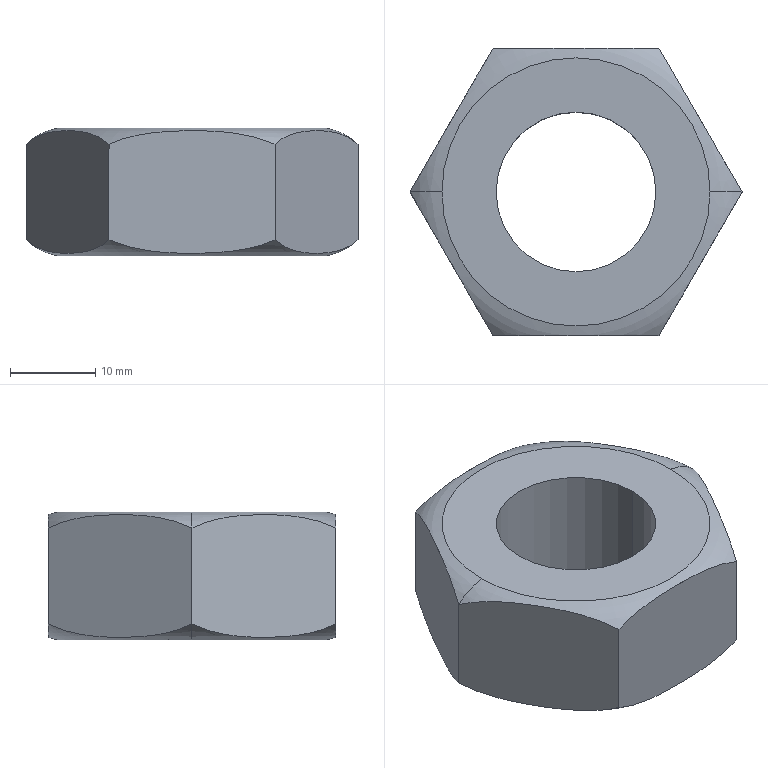Part | SolidWorks | features Extrusion 1, RevCut 1, Scale 1 | 1 solid | 14 faces | box 38.971 x 33.75 x 15 mm | volume 10501 mm3 | plane 8 | torus 4 | cylinder 2 | commonest cylinder face diameters 18.75 x2
STEP:
#1=CARTESIAN_POINT('',(-15.736,-0.00008146,11.5));
#2=VERTEX_POINT('',#1);
#3=CARTESIAN_POINT('',(15.736,-0.00008146,11.5));
#4=VERTEX_POINT('',#3);
#5=CARTESIAN_POINT('',(0.00005689,-0.00008146,11.5));
#6=DIRECTION('',(0.,0.,-1.));
#7=DIRECTION('',(-1.,0.,0.));
#8=AXIS2_PLACEMENT_3D('',#5,#6,#7);
#9=CIRCLE('',#8,15.736);
#10=EDGE_CURVE('',#2,#4,#9,.T.);
#11=ORIENTED_EDGE('',*,*,#10,.T.);
#12=CARTESIAN_POINT('',(19.486,-0.00008146,9.625));
#13=VERTEX_POINT('',#12);
#14=CARTESIAN_POINT('',(14.39,-0.00008146,4.122));
#15=DIRECTION('',(0.,1.,0.));
#16=DIRECTION('',(-1.,0.,0.));
#17=AXIS2_PLACEMENT_3D('',#14,#15,#16);
#18=CIRCLE('',#17,7.5);
#19=EDGE_CURVE('',#4,#13,#18,.T.);
#20=ORIENTED_EDGE('',*,*,#19,.T.);
#21=CARTESIAN_POINT('',(9.743,16.875,9.625));
#22=VERTEX_POINT('',#21);
#23=CARTESIAN_POINT('',(9.743,16.875,9.625));
#24=CARTESIAN_POINT('',(10.123,16.216,9.977));
#25=CARTESIAN_POINT('',(10.516,15.536,10.239));
#26=CARTESIAN_POINT('',(11.316,14.15,10.649));
#27=CARTESIAN_POINT('',(11.724,13.444,10.796));
#28=CARTESIAN_POINT('',(12.549,12.014,11.016));
#29=CARTESIAN_POINT('',(12.962,11.298,11.086));
#30=CARTESIAN_POINT('',(13.788,9.869,11.177));
#31=CARTESIAN_POINT('',(14.2,9.155,11.198));
#32=CARTESIAN_POINT('',(15.024,7.728,11.198));
#33=CARTESIAN_POINT('',(15.436,7.014,11.178));
#34=CARTESIAN_POINT('',(16.259,5.588,11.087));
#35=CARTESIAN_POINT('',(16.671,4.876,11.017));
#36=CARTESIAN_POINT('',(17.493,3.452,10.8));
#37=CARTESIAN_POINT('',(17.905,2.737,10.652));
#38=CARTESIAN_POINT('',(18.711,1.341,10.24));
#39=CARTESIAN_POINT('',(19.105,0.6588,9.977));
#40=CARTESIAN_POINT('',(19.486,-0.00008146,9.625));
#41=B_SPLINE_CURVE_WITH_KNOTS('',3,(#23,#24,#25,#26,#27,#28,#29,#30,#31,#32,#33,#34,#35,#36,#37,#38,#39,#40),.UNSPECIFIED.,.F.,.F.,(4,2,2,2,2,2,2,2,4),(0.00000047,0.002478,0.004956,0.007434,0.009912,0.01239,0.01487,0.01735,0.01982),.UNSPECIFIED.);
#42=EDGE_CURVE('',#22,#13,#41,.T.);
#43=ORIENTED_EDGE('',*,*,#42,.F.);
#44=CARTESIAN_POINT('',(-9.743,16.875,9.625));
#45=VERTEX_POINT('',#44);
#46=CARTESIAN_POINT('',(-9.743,16.875,9.625));
#47=CARTESIAN_POINT('',(-8.991,16.875,9.973));
#48=CARTESIAN_POINT('',(-8.209,16.875,10.235));
#49=CARTESIAN_POINT('',(-7.003,16.875,10.545));
#50=CARTESIAN_POINT('',(-6.595,16.875,10.634));
#51=CARTESIAN_POINT('',(-5.78,16.875,10.787));
#52=CARTESIAN_POINT('',(-5.371,16.875,10.851));
#53=CARTESIAN_POINT('',(-4.142,16.875,11.014));
#54=CARTESIAN_POINT('',(-3.319,16.875,11.085));
#55=CARTESIAN_POINT('',(-1.669,16.875,11.177));
#56=CARTESIAN_POINT('',(-0.841,16.875,11.198));
#57=CARTESIAN_POINT('',(0.8178,16.875,11.198));
#58=CARTESIAN_POINT('',(1.647,16.875,11.178));
#59=CARTESIAN_POINT('',(3.299,16.875,11.087));
#60=CARTESIAN_POINT('',(4.122,16.875,11.016));
#61=CARTESIAN_POINT('',(5.76,16.875,10.8));
#62=CARTESIAN_POINT('',(6.575,16.875,10.654));
#63=CARTESIAN_POINT('',(7.788,16.875,10.344));
#64=CARTESIAN_POINT('',(8.19,16.875,10.226));
#65=CARTESIAN_POINT('',(8.977,16.875,9.954));
#66=CARTESIAN_POINT('',(9.364,16.875,9.8));
#67=CARTESIAN_POINT('',(9.743,16.875,9.625));
#68=B_SPLINE_CURVE_WITH_KNOTS('',3,(#46,#47,#48,#49,#50,#51,#52,#53,#54,#55,#56,#57,#58,#59,#60,#61,#62,#63,#64,#65,#66,#67),.UNSPECIFIED.,.F.,.F.,(4,2,2,2,2,2,2,2,2,2,4),(0.05874,0.06121,0.06245,0.06369,0.06617,0.06865,0.07112,0.0736,0.07608,0.07732,0.07856),.UNSPECIFIED.);
#69=EDGE_CURVE('',#45,#22,#68,.T.);
#70=ORIENTED_EDGE('',*,*,#69,.F.);
#71=CARTESIAN_POINT('',(-19.486,-0.00008146,9.625));
#72=VERTEX_POINT('',#71);
#73=CARTESIAN_POINT('',(-19.486,-0.00008146,9.625));
#74=CARTESIAN_POINT('',(-19.105,0.6591,9.977));
#75=CARTESIAN_POINT('',(-18.712,1.339,10.239));
#76=CARTESIAN_POINT('',(-17.912,2.725,10.649));
#77=CARTESIAN_POINT('',(-17.504,3.431,10.796));
#78=CARTESIAN_POINT('',(-16.679,4.861,11.016));
#79=CARTESIAN_POINT('',(-16.266,5.577,11.086));
#80=CARTESIAN_POINT('',(-15.441,7.006,11.177));
#81=CARTESIAN_POINT('',(-15.029,7.72,11.198));
#82=CARTESIAN_POINT('',(-14.204,9.147,11.198));
#83=CARTESIAN_POINT('',(-13.792,9.861,11.178));
#84=CARTESIAN_POINT('',(-12.969,11.287,11.087));
#85=CARTESIAN_POINT('',(-12.558,11.999,11.017));
#86=CARTESIAN_POINT('',(-11.736,13.423,10.8));
#87=CARTESIAN_POINT('',(-11.323,14.138,10.652));
#88=CARTESIAN_POINT('',(-10.517,15.533,10.24));
#89=CARTESIAN_POINT('',(-10.123,16.216,9.977));
#90=CARTESIAN_POINT('',(-9.743,16.875,9.625));
#91=B_SPLINE_CURVE_WITH_KNOTS('',3,(#73,#74,#75,#76,#77,#78,#79,#80,#81,#82,#83,#84,#85,#86,#87,#88,#89,#90),.UNSPECIFIED.,.F.,.F.,(4,2,2,2,2,2,2,2,4),(0.00000047,0.002478,0.004956,0.007434,0.009912,0.01239,0.01487,0.01735,0.01982),.UNSPECIFIED.);
#92=EDGE_CURVE('',#72,#45,#91,.T.);
#93=ORIENTED_EDGE('',*,*,#92,.F.);
#94=CARTESIAN_POINT('',(-14.39,-0.00008146,4.122));
#95=DIRECTION('',(0.,-1.,0.));
#96=DIRECTION('',(0.,0.,-1.));
#97=AXIS2_PLACEMENT_3D('',#94,#95,#96);
#98=CIRCLE('',#97,7.5);
#99=EDGE_CURVE('',#2,#72,#98,.T.);
#100=ORIENTED_EDGE('',*,*,#99,.F.);
#101=EDGE_LOOP('',(#11,#20,#43,#70,#93,#100));
#102=FACE_OUTER_BOUND('',#101,.T.);
#103=CARTESIAN_POINT('',(0.00005689,-0.00008146,4.122));
#104=DIRECTION('',(0.,0.,-1.));
#105=DIRECTION('',(-1.,0.,0.));
#106=AXIS2_PLACEMENT_3D('',#103,#104,#105);
#107=TOROIDAL_SURFACE('',#106,14.39,7.5);
#108=ADVANCED_FACE('',(#102),#107,.T.);
#109=CARTESIAN_POINT('',(19.486,-0.00008146,-1.625));
#110=VERTEX_POINT('',#109);
#111=CARTESIAN_POINT('',(9.743,16.875,-1.625));
#112=VERTEX_POINT('',#111);
#113=CARTESIAN_POINT('',(19.486,-0.00008146,-1.625));
#114=CARTESIAN_POINT('',(19.105,0.6591,-1.977));
#115=CARTESIAN_POINT('',(18.712,1.339,-2.239));
#116=CARTESIAN_POINT('',(17.912,2.725,-2.649));
#117=CARTESIAN_POINT('',(17.505,3.431,-2.796));
#118=CARTESIAN_POINT('',(16.679,4.861,-3.016));
#119=CARTESIAN_POINT('',(16.266,5.577,-3.086));
#120=CARTESIAN_POINT('',(15.441,7.006,-3.177));
#121=CARTESIAN_POINT('',(15.029,7.72,-3.198));
#122=CARTESIAN_POINT('',(14.204,9.147,-3.198));
#123=CARTESIAN_POINT('',(13.793,9.861,-3.178));
#124=CARTESIAN_POINT('',(12.969,11.287,-3.087));
#125=CARTESIAN_POINT('',(12.558,11.999,-3.017));
#126=CARTESIAN_POINT('',(11.736,13.423,-2.8));
#127=CARTESIAN_POINT('',(11.323,14.138,-2.652));
#128=CARTESIAN_POINT('',(10.517,15.533,-2.24));
#129=CARTESIAN_POINT('',(10.123,16.216,-1.977));
#130=CARTESIAN_POINT('',(9.743,16.875,-1.625));
#131=B_SPLINE_CURVE_WITH_KNOTS('',3,(#113,#114,#115,#116,#117,#118,#119,#120,#121,#122,#123,#124,#125,#126,#127,#128,#129,#130),.UNSPECIFIED.,.F.,.F.,(4,2,2,2,2,2,2,2,4),(0.00000047,0.002478,0.004956,0.007434,0.009912,0.01239,0.01487,0.01735,0.01982),.UNSPECIFIED.);
#132=EDGE_CURVE('',#110,#112,#131,.T.);
#133=ORIENTED_EDGE('',*,*,#132,.F.);
#134=CARTESIAN_POINT('',(15.736,-0.00008146,-3.5));
#135=VERTEX_POINT('',#134);
#136=CARTESIAN_POINT('',(14.39,-0.00008146,3.878));
#137=DIRECTION('',(0.,1.,0.));
#138=DIRECTION('',(-1.,0.,0.));
#139=AXIS2_PLACEMENT_3D('',#136,#137,#138);
#140=CIRCLE('',#139,7.5);
#141=EDGE_CURVE('',#110,#135,#140,.T.);
#142=ORIENTED_EDGE('',*,*,#141,.T.);
#143=CARTESIAN_POINT('',(-15.736,-0.00008146,-3.5));
#144=VERTEX_POINT('',#143);
#145=CARTESIAN_POINT('',(0.00005689,-0.00008146,-3.5));
#146=DIRECTION('',(0.,0.,-1.));
#147=DIRECTION('',(-1.,0.,0.));
#148=AXIS2_PLACEMENT_3D('',#145,#146,#147);
#149=CIRCLE('',#148,15.736);
#150=EDGE_CURVE('',#144,#135,#149,.T.);
#151=ORIENTED_EDGE('',*,*,#150,.F.);
#152=CARTESIAN_POINT('',(-19.486,-0.00008146,-1.625));
#153=VERTEX_POINT('',#152);
#154=CARTESIAN_POINT('',(-14.39,-0.00008146,3.878));
#155=DIRECTION('',(0.,-1.,0.));
#156=DIRECTION('',(0.,0.,-1.));
#157=AXIS2_PLACEMENT_3D('',#154,#155,#156);
#158=CIRCLE('',#157,7.5);
#159=EDGE_CURVE('',#153,#144,#158,.T.);
#160=ORIENTED_EDGE('',*,*,#159,.F.);
#161=CARTESIAN_POINT('',(-9.743,16.875,-1.625));
#162=VERTEX_POINT('',#161);
#163=CARTESIAN_POINT('',(-9.743,16.875,-1.625));
#164=CARTESIAN_POINT('',(-10.123,16.216,-1.977));
#165=CARTESIAN_POINT('',(-10.516,15.536,-2.239));
#166=CARTESIAN_POINT('',(-11.316,14.15,-2.649));
#167=CARTESIAN_POINT('',(-11.724,13.444,-2.796));
#168=CARTESIAN_POINT('',(-12.549,12.014,-3.016));
#169=CARTESIAN_POINT('',(-12.962,11.298,-3.086));
#170=CARTESIAN_POINT('',(-13.787,9.869,-3.177));
#171=CARTESIAN_POINT('',(-14.2,9.155,-3.198));
#172=CARTESIAN_POINT('',(-15.024,7.728,-3.198));
#173=CARTESIAN_POINT('',(-15.436,7.014,-3.178));
#174=CARTESIAN_POINT('',(-16.259,5.588,-3.087));
#175=CARTESIAN_POINT('',(-16.67,4.876,-3.017));
#176=CARTESIAN_POINT('',(-17.492,3.452,-2.8));
#177=CARTESIAN_POINT('',(-17.905,2.737,-2.652));
#178=CARTESIAN_POINT('',(-18.711,1.341,-2.24));
#179=CARTESIAN_POINT('',(-19.105,0.6588,-1.977));
#180=CARTESIAN_POINT('',(-19.486,-0.00008146,-1.625));
#181=B_SPLINE_CURVE_WITH_KNOTS('',3,(#163,#164,#165,#166,#167,#168,#169,#170,#171,#172,#173,#174,#175,#176,#177,#178,#179,#180),.UNSPECIFIED.,.F.,.F.,(4,2,2,2,2,2,2,2,4),(0.00000047,0.002478,0.004956,0.007434,0.009912,0.01239,0.01487,0.01735,0.01982),.UNSPECIFIED.);
#182=EDGE_CURVE('',#162,#153,#181,.T.);
#183=ORIENTED_EDGE('',*,*,#182,.F.);
#184=CARTESIAN_POINT('',(9.743,16.875,-1.625));
#185=CARTESIAN_POINT('',(8.992,16.875,-1.973));
#186=CARTESIAN_POINT('',(8.209,16.875,-2.235));
#187=CARTESIAN_POINT('',(7.003,16.875,-2.545));
#188=CARTESIAN_POINT('',(6.596,16.875,-2.634));
#189=CARTESIAN_POINT('',(5.78,16.875,-2.786));
#190=CARTESIAN_POINT('',(5.371,16.875,-2.851));
#191=CARTESIAN_POINT('',(4.142,16.875,-3.014));
#192=CARTESIAN_POINT('',(3.319,16.875,-3.085));
#193=CARTESIAN_POINT('',(1.669,16.875,-3.177));
#194=CARTESIAN_POINT('',(0.8411,16.875,-3.198));
#195=CARTESIAN_POINT('',(-0.8176,16.875,-3.198));
#196=CARTESIAN_POINT('',(-1.647,16.875,-3.178));
#197=CARTESIAN_POINT('',(-3.299,16.875,-3.087));
#198=CARTESIAN_POINT('',(-4.122,16.875,-3.016));
#199=CARTESIAN_POINT('',(-5.76,16.875,-2.8));
#200=CARTESIAN_POINT('',(-6.575,16.875,-2.654));
#201=CARTESIAN_POINT('',(-7.788,16.875,-2.344));
#202=CARTESIAN_POINT('',(-8.189,16.875,-2.226));
#203=CARTESIAN_POINT('',(-8.977,16.875,-1.954));
#204=CARTESIAN_POINT('',(-9.364,16.875,-1.8));
#205=CARTESIAN_POINT('',(-9.743,16.875,-1.625));
#206=B_SPLINE_CURVE_WITH_KNOTS('',3,(#184,#185,#186,#187,#188,#189,#190,#191,#192,#193,#194,#195,#196,#197,#198,#199,#200,#201,#202,#203,#204,#205),.UNSPECIFIED.,.F.,.F.,(4,2,2,2,2,2,2,2,2,2,4),(0.05874,0.06121,0.06245,0.06369,0.06617,0.06865,0.07112,0.0736,0.07608,0.07732,0.07856),.UNSPECIFIED.);
#207=EDGE_CURVE('',#112,#162,#206,.T.);
#208=ORIENTED_EDGE('',*,*,#207,.F.);
#209=EDGE_LOOP('',(#133,#142,#151,#160,#183,#208));
#210=FACE_OUTER_BOUND('',#209,.T.);
#211=CARTESIAN_POINT('',(0.00005689,-0.00008146,3.878));
#212=DIRECTION('',(0.,0.,-1.));
#213=DIRECTION('',(-1.,0.,0.));
#214=AXIS2_PLACEMENT_3D('',#211,#212,#213);
#215=TOROIDAL_SURFACE('',#214,14.39,7.5);
#216=ADVANCED_FACE('',(#210),#215,.T.);
#217=CARTESIAN_POINT('',(-9.375,-0.00008146,11.5));
#218=VERTEX_POINT('',#217);
#219=CARTESIAN_POINT('',(9.375,-0.00008146,11.5));
#220=VERTEX_POINT('',#219);
#221=CARTESIAN_POINT('',(0.00005689,-0.00008146,11.5));
#222=DIRECTION('',(0.,0.,1.));
#223=DIRECTION('',(1.,0.,0.));
#224=AXIS2_PLACEMENT_3D('',#221,#222,#223);
#225=CIRCLE('',#224,9.375);
#226=EDGE_CURVE('',#218,#220,#225,.T.);
#227=ORIENTED_EDGE('',*,*,#226,.T.);
#228=CARTESIAN_POINT('',(9.375,-0.00008146,-3.5));
#229=VERTEX_POINT('',#228);
#230=CARTESIAN_POINT('',(9.375,-0.00008146,11.5));
#231=DIRECTION('',(0.,0.,-1.));
#232=VECTOR('',#231,1000.);
#233=LINE('',#230,#232);
#234=EDGE_CURVE('',#220,#229,#233,.T.);
#235=ORIENTED_EDGE('',*,*,#234,.T.);
#236=CARTESIAN_POINT('',(-9.375,-0.00008146,-3.5));
#237=VERTEX_POINT('',#236);
#238=CARTESIAN_POINT('',(0.00005689,-0.00008146,-3.5));
#239=DIRECTION('',(0.,0.,1.));
#240=DIRECTION('',(1.,0.,0.));
#241=AXIS2_PLACEMENT_3D('',#238,#239,#240);
#242=CIRCLE('',#241,9.375);
#243=EDGE_CURVE('',#237,#229,#242,.T.);
#244=ORIENTED_EDGE('',*,*,#243,.F.);
#245=CARTESIAN_POINT('',(-9.375,-0.00008146,11.5));
#246=DIRECTION('',(0.,0.,-1.));
#247=VECTOR('',#246,1000.);
#248=LINE('',#245,#247);
#249=EDGE_CURVE('',#218,#237,#248,.T.);
#250=ORIENTED_EDGE('',*,*,#249,.F.);
#251=EDGE_LOOP('',(#227,#235,#244,#250));
#252=FACE_OUTER_BOUND('',#251,.T.);
#253=CARTESIAN_POINT('',(0.00005689,-0.00008146,11.5));
#254=DIRECTION('',(0.,0.,-1.));
#255=DIRECTION('',(-1.,0.,0.));
#256=AXIS2_PLACEMENT_3D('',#253,#254,#255);
#257=CYLINDRICAL_SURFACE('',#256,9.375);
#258=ADVANCED_FACE('',(#252),#257,.F.);
#259=ORIENTED_EDGE('',*,*,#10,.F.);
#260=CARTESIAN_POINT('',(0.00005689,-0.00008146,11.5));
#261=DIRECTION('',(0.,0.,-1.));
#262=DIRECTION('',(-1.,0.,0.));
#263=AXIS2_PLACEMENT_3D('',#260,#261,#262);
#264=CIRCLE('',#263,15.736);
#265=EDGE_CURVE('',#4,#2,#264,.T.);
#266=ORIENTED_EDGE('',*,*,#265,.F.);
#267=EDGE_LOOP('',(#259,#266));
#268=FACE_OUTER_BOUND('',#267,.T.);
#269=ORIENTED_EDGE('',*,*,#226,.F.);
#270=CARTESIAN_POINT('',(0.00005689,-0.00008146,11.5));
#271=DIRECTION('',(0.,0.,1.));
#272=DIRECTION('',(1.,0.,0.));
#273=AXIS2_PLACEMENT_3D('',#270,#271,#272);
#274=CIRCLE('',#273,9.375);
#275=EDGE_CURVE('',#220,#218,#274,.T.);
#276=ORIENTED_EDGE('',*,*,#275,.F.);
#277=EDGE_LOOP('',(#269,#276));
#278=FACE_BOUND('',#277,.T.);
#279=CARTESIAN_POINT('',(0.00005689,-0.00008146,11.5));
#280=DIRECTION('',(0.,0.,1.));
#281=DIRECTION('',(1.,0.,0.));
#282=AXIS2_PLACEMENT_3D('',#279,#280,#281);
#283=PLANE('',#282);
#284=ADVANCED_FACE('',(#268,#278),#283,.T.);
#285=ORIENTED_EDGE('',*,*,#150,.T.);
#286=CARTESIAN_POINT('',(0.00005689,-0.00008146,-3.5));
#287=DIRECTION('',(0.,0.,-1.));
#288=DIRECTION('',(-1.,0.,0.));
#289=AXIS2_PLACEMENT_3D('',#286,#287,#288);
#290=CIRCLE('',#289,15.736);
#291=EDGE_CURVE('',#135,#144,#290,.T.);
#292=ORIENTED_EDGE('',*,*,#291,.T.);
#293=EDGE_LOOP('',(#285,#292));
#294=FACE_OUTER_BOUND('',#293,.T.);
#295=ORIENTED_EDGE('',*,*,#243,.T.);
#296=CARTESIAN_POINT('',(0.00005689,-0.00008146,-3.5));
#297=DIRECTION('',(0.,0.,1.));
#298=DIRECTION('',(1.,0.,0.));
#299=AXIS2_PLACEMENT_3D('',#296,#297,#298);
#300=CIRCLE('',#299,9.375);
#301=EDGE_CURVE('',#229,#237,#300,.T.);
#302=ORIENTED_EDGE('',*,*,#301,.T.);
#303=EDGE_LOOP('',(#295,#302));
#304=FACE_BOUND('',#303,.T.);
#305=CARTESIAN_POINT('',(0.00005689,-0.00008146,-3.5));
#306=DIRECTION('',(0.,0.,1.));
#307=DIRECTION('',(1.,0.,0.));
#308=AXIS2_PLACEMENT_3D('',#305,#306,#307);
#309=PLANE('',#308);
#310=ADVANCED_FACE('',(#294,#304),#309,.F.);
#311=CARTESIAN_POINT('',(19.486,-0.00008146,11.5));
#312=DIRECTION('',(0.,0.,-1.));
#313=VECTOR('',#312,1000.);
#314=LINE('',#311,#313);
#315=EDGE_CURVE('',#13,#110,#314,.T.);
#316=ORIENTED_EDGE('',*,*,#315,.F.);
#317=CARTESIAN_POINT('',(9.743,-16.875,9.625));
#318=VERTEX_POINT('',#317);
#319=CARTESIAN_POINT('',(19.486,-0.00008146,9.625));
#320=CARTESIAN_POINT('',(19.105,-0.6593,9.977));
#321=CARTESIAN_POINT('',(18.712,-1.339,10.239));
#322=CARTESIAN_POINT('',(17.912,-2.725,10.649));
#323=CARTESIAN_POINT('',(17.505,-3.431,10.796));
#324=CARTESIAN_POINT('',(16.679,-4.861,11.016));
#325=CARTESIAN_POINT('',(16.266,-5.577,11.086));
#326=CARTESIAN_POINT('',(15.441,-7.006,11.177));
#327=CARTESIAN_POINT('',(15.029,-7.72,11.198));
#328=CARTESIAN_POINT('',(14.204,-9.147,11.198));
#329=CARTESIAN_POINT('',(13.793,-9.861,11.178));
#330=CARTESIAN_POINT('',(12.969,-11.287,11.087));
#331=CARTESIAN_POINT('',(12.558,-11.999,11.017));
#332=CARTESIAN_POINT('',(11.736,-13.423,10.8));
#333=CARTESIAN_POINT('',(11.323,-14.138,10.652));
#334=CARTESIAN_POINT('',(10.517,-15.534,10.24));
#335=CARTESIAN_POINT('',(10.123,-16.216,9.977));
#336=CARTESIAN_POINT('',(9.743,-16.875,9.625));
#337=B_SPLINE_CURVE_WITH_KNOTS('',3,(#319,#320,#321,#322,#323,#324,#325,#326,#327,#328,#329,#330,#331,#332,#333,#334,#335,#336),.UNSPECIFIED.,.F.,.F.,(4,2,2,2,2,2,2,2,4),(0.00000047,0.002478,0.004956,0.007434,0.009912,0.01239,0.01487,0.01735,0.01982),.UNSPECIFIED.);
#338=EDGE_CURVE('',#13,#318,#337,.T.);
#339=ORIENTED_EDGE('',*,*,#338,.T.);
#340=CARTESIAN_POINT('',(9.743,-16.875,-1.625));
#341=VERTEX_POINT('',#340);
#342=CARTESIAN_POINT('',(9.743,-16.875,11.5));
#343=DIRECTION('',(0.,0.,-1.));
#344=VECTOR('',#343,1000.);
#345=LINE('',#342,#344);
#346=EDGE_CURVE('',#318,#341,#345,.T.);
#347=ORIENTED_EDGE('',*,*,#346,.T.);
#348=CARTESIAN_POINT('',(9.743,-16.875,-1.625));
#349=CARTESIAN_POINT('',(10.123,-16.216,-1.977));
#350=CARTESIAN_POINT('',(10.516,-15.536,-2.239));
#351=CARTESIAN_POINT('',(11.316,-14.15,-2.649));
#352=CARTESIAN_POINT('',(11.724,-13.444,-2.796));
#353=CARTESIAN_POINT('',(12.549,-12.014,-3.016));
#354=CARTESIAN_POINT('',(12.962,-11.298,-3.086));
#355=CARTESIAN_POINT('',(13.788,-9.869,-3.177));
#356=CARTESIAN_POINT('',(14.2,-9.155,-3.198));
#357=CARTESIAN_POINT('',(15.024,-7.728,-3.198));
#358=CARTESIAN_POINT('',(15.436,-7.014,-3.178));
#359=CARTESIAN_POINT('',(16.259,-5.588,-3.087));
#360=CARTESIAN_POINT('',(16.671,-4.876,-3.017));
#361=CARTESIAN_POINT('',(17.493,-3.452,-2.8));
#362=CARTESIAN_POINT('',(17.905,-2.737,-2.652));
#363=CARTESIAN_POINT('',(18.711,-1.342,-2.24));
#364=CARTESIAN_POINT('',(19.105,-0.659,-1.977));
#365=CARTESIAN_POINT('',(19.486,-0.00008146,-1.625));
#366=B_SPLINE_CURVE_WITH_KNOTS('',3,(#348,#349,#350,#351,#352,#353,#354,#355,#356,#357,#358,#359,#360,#361,#362,#363,#364,#365),.UNSPECIFIED.,.F.,.F.,(4,2,2,2,2,2,2,2,4),(0.00000047,0.002478,0.004956,0.007434,0.009912,0.01239,0.01487,0.01735,0.01982),.UNSPECIFIED.);
#367=EDGE_CURVE('',#341,#110,#366,.T.);
#368=ORIENTED_EDGE('',*,*,#367,.T.);
#369=EDGE_LOOP('',(#316,#339,#347,#368));
#370=FACE_OUTER_BOUND('',#369,.T.);
#371=CARTESIAN_POINT('',(9.743,-16.875,11.5));
#372=DIRECTION('',(-0.866,0.5,0.));
#373=DIRECTION('',(-0.5,-0.866,0.));
#374=AXIS2_PLACEMENT_3D('',#371,#372,#373);
#375=PLANE('',#374);
#376=ADVANCED_FACE('',(#370),#375,.F.);
#377=CARTESIAN_POINT('',(9.743,16.875,11.5));
#378=DIRECTION('',(0.,0.,-1.));
#379=VECTOR('',#378,1000.);
#380=LINE('',#377,#379);
#381=EDGE_CURVE('',#22,#112,#380,.T.);
#382=ORIENTED_EDGE('',*,*,#381,.F.);
#383=ORIENTED_EDGE('',*,*,#42,.T.);
#384=ORIENTED_EDGE('',*,*,#315,.T.);
#385=ORIENTED_EDGE('',*,*,#132,.T.);
#386=EDGE_LOOP('',(#382,#383,#384,#385));
#387=FACE_OUTER_BOUND('',#386,.T.);
#388=CARTESIAN_POINT('',(19.486,-0.00008146,11.5));
#389=DIRECTION('',(-0.866,-0.5,0.));
#390=DIRECTION('',(0.5,-0.866,0.));
#391=AXIS2_PLACEMENT_3D('',#388,#389,#390);
#392=PLANE('',#391);
#393=ADVANCED_FACE('',(#387),#392,.F.);
#394=CARTESIAN_POINT('',(-9.743,16.875,11.5));
#395=DIRECTION('',(0.,0.,-1.));
#396=VECTOR('',#395,1000.);
#397=LINE('',#394,#396);
#398=EDGE_CURVE('',#45,#162,#397,.T.);
#399=ORIENTED_EDGE('',*,*,#398,.F.);
#400=ORIENTED_EDGE('',*,*,#69,.T.);
#401=ORIENTED_EDGE('',*,*,#381,.T.);
#402=ORIENTED_EDGE('',*,*,#207,.T.);
#403=EDGE_LOOP('',(#399,#400,#401,#402));
#404=FACE_OUTER_BOUND('',#403,.T.);
#405=CARTESIAN_POINT('',(9.743,16.875,11.5));
#406=DIRECTION('',(0.,-1.,0.));
#407=DIRECTION('',(0.,0.,-1.));
#408=AXIS2_PLACEMENT_3D('',#405,#406,#407);
#409=PLANE('',#408);
#410=ADVANCED_FACE('',(#404),#409,.F.);
#411=CARTESIAN_POINT('',(-19.486,-0.00008146,11.5));
#412=DIRECTION('',(0.,0.,-1.));
#413=VECTOR('',#412,1000.);
#414=LINE('',#411,#413);
#415=EDGE_CURVE('',#72,#153,#414,.T.);
#416=ORIENTED_EDGE('',*,*,#415,.F.);
#417=ORIENTED_EDGE('',*,*,#92,.T.);
#418=ORIENTED_EDGE('',*,*,#398,.T.);
#419=ORIENTED_EDGE('',*,*,#182,.T.);
#420=EDGE_LOOP('',(#416,#417,#418,#419));
#421=FACE_OUTER_BOUND('',#420,.T.);
#422=CARTESIAN_POINT('',(-9.743,16.875,11.5));
#423=DIRECTION('',(0.866,-0.5,0.));
#424=DIRECTION('',(0.5,0.866,0.));
#425=AXIS2_PLACEMENT_3D('',#422,#423,#424);
#426=PLANE('',#425);
#427=ADVANCED_FACE('',(#421),#426,.F.);
#428=CARTESIAN_POINT('',(-9.743,-16.875,9.625));
#429=VERTEX_POINT('',#428);
#430=CARTESIAN_POINT('',(-9.743,-16.875,-1.625));
#431=VERTEX_POINT('',#430);
#432=CARTESIAN_POINT('',(-9.743,-16.875,11.5));
#433=DIRECTION('',(0.,0.,-1.));
#434=VECTOR('',#433,1000.);
#435=LINE('',#432,#434);
#436=EDGE_CURVE('',#429,#431,#435,.T.);
#437=ORIENTED_EDGE('',*,*,#436,.F.);
#438=CARTESIAN_POINT('',(-9.743,-16.875,9.625));
#439=CARTESIAN_POINT('',(-10.123,-16.216,9.977));
#440=CARTESIAN_POINT('',(-10.516,-15.536,10.239));
#441=CARTESIAN_POINT('',(-11.316,-14.15,10.649));
#442=CARTESIAN_POINT('',(-11.724,-13.444,10.796));
#443=CARTESIAN_POINT('',(-12.549,-12.014,11.016));
#444=CARTESIAN_POINT('',(-12.962,-11.298,11.086));
#445=CARTESIAN_POINT('',(-13.787,-9.869,11.177));
#446=CARTESIAN_POINT('',(-14.2,-9.155,11.198));
#447=CARTESIAN_POINT('',(-15.024,-7.728,11.198));
#448=CARTESIAN_POINT('',(-15.436,-7.014,11.178));
#449=CARTESIAN_POINT('',(-16.259,-5.588,11.087));
#450=CARTESIAN_POINT('',(-16.67,-4.876,11.017));
#451=CARTESIAN_POINT('',(-17.492,-3.452,10.8));
#452=CARTESIAN_POINT('',(-17.905,-2.737,10.652));
#453=CARTESIAN_POINT('',(-18.711,-1.342,10.24));
#454=CARTESIAN_POINT('',(-19.105,-0.659,9.977));
#455=CARTESIAN_POINT('',(-19.486,-0.00008146,9.625));
#456=B_SPLINE_CURVE_WITH_KNOTS('',3,(#438,#439,#440,#441,#442,#443,#444,#445,#446,#447,#448,#449,#450,#451,#452,#453,#454,#455),.UNSPECIFIED.,.F.,.F.,(4,2,2,2,2,2,2,2,4),(0.00000047,0.002478,0.004956,0.007434,0.009912,0.01239,0.01487,0.01735,0.01982),.UNSPECIFIED.);
#457=EDGE_CURVE('',#429,#72,#456,.T.);
#458=ORIENTED_EDGE('',*,*,#457,.T.);
#459=ORIENTED_EDGE('',*,*,#415,.T.);
#460=CARTESIAN_POINT('',(-19.486,-0.00008146,-1.625));
#461=CARTESIAN_POINT('',(-19.105,-0.6593,-1.977));
#462=CARTESIAN_POINT('',(-18.712,-1.339,-2.239));
#463=CARTESIAN_POINT('',(-17.912,-2.725,-2.649));
#464=CARTESIAN_POINT('',(-17.504,-3.431,-2.796));
#465=CARTESIAN_POINT('',(-16.679,-4.861,-3.016));
#466=CARTESIAN_POINT('',(-16.266,-5.577,-3.086));
#467=CARTESIAN_POINT('',(-15.441,-7.006,-3.177));
#468=CARTESIAN_POINT('',(-15.029,-7.72,-3.198));
#469=CARTESIAN_POINT('',(-14.204,-9.147,-3.198));
#470=CARTESIAN_POINT('',(-13.792,-9.861,-3.178));
#471=CARTESIAN_POINT('',(-12.969,-11.287,-3.087));
#472=CARTESIAN_POINT('',(-12.558,-11.999,-3.017));
#473=CARTESIAN_POINT('',(-11.736,-13.423,-2.8));
#474=CARTESIAN_POINT('',(-11.323,-14.138,-2.652));
#475=CARTESIAN_POINT('',(-10.517,-15.534,-2.24));
#476=CARTESIAN_POINT('',(-10.123,-16.216,-1.977));
#477=CARTESIAN_POINT('',(-9.743,-16.875,-1.625));
#478=B_SPLINE_CURVE_WITH_KNOTS('',3,(#460,#461,#462,#463,#464,#465,#466,#467,#468,#469,#470,#471,#472,#473,#474,#475,#476,#477),.UNSPECIFIED.,.F.,.F.,(4,2,2,2,2,2,2,2,4),(0.00000047,0.002478,0.004956,0.007434,0.009912,0.01239,0.01487,0.01735,0.01982),.UNSPECIFIED.);
#479=EDGE_CURVE('',#153,#431,#478,.T.);
#480=ORIENTED_EDGE('',*,*,#479,.T.);
#481=EDGE_LOOP('',(#437,#458,#459,#480));
#482=FACE_OUTER_BOUND('',#481,.T.);
#483=CARTESIAN_POINT('',(-19.486,-0.00008146,11.5));
#484=DIRECTION('',(0.866,0.5,0.));
#485=DIRECTION('',(-0.5,0.866,0.));
#486=AXIS2_PLACEMENT_3D('',#483,#484,#485);
#487=PLANE('',#486);
#488=ADVANCED_FACE('',(#482),#487,.F.);
#489=ORIENTED_EDGE('',*,*,#346,.F.);
#490=CARTESIAN_POINT('',(9.743,-16.875,9.625));
#491=CARTESIAN_POINT('',(8.992,-16.875,9.973));
#492=CARTESIAN_POINT('',(8.209,-16.875,10.235));
#493=CARTESIAN_POINT('',(7.003,-16.875,10.545));
#494=CARTESIAN_POINT('',(6.596,-16.875,10.634));
#495=CARTESIAN_POINT('',(5.78,-16.875,10.787));
#496=CARTESIAN_POINT('',(5.371,-16.875,10.851));
#497=CARTESIAN_POINT('',(4.142,-16.875,11.014));
#498=CARTESIAN_POINT('',(3.319,-16.875,11.085));
#499=CARTESIAN_POINT('',(1.669,-16.875,11.177));
#500=CARTESIAN_POINT('',(0.8411,-16.875,11.198));
#501=CARTESIAN_POINT('',(-0.8176,-16.875,11.198));
#502=CARTESIAN_POINT('',(-1.647,-16.875,11.178));
#503=CARTESIAN_POINT('',(-3.299,-16.875,11.087));
#504=CARTESIAN_POINT('',(-4.122,-16.875,11.016));
#505=CARTESIAN_POINT('',(-5.76,-16.875,10.8));
#506=CARTESIAN_POINT('',(-6.575,-16.875,10.654));
#507=CARTESIAN_POINT('',(-7.788,-16.875,10.344));
#508=CARTESIAN_POINT('',(-8.189,-16.875,10.226));
#509=CARTESIAN_POINT('',(-8.977,-16.875,9.954));
#510=CARTESIAN_POINT('',(-9.364,-16.875,9.8));
#511=CARTESIAN_POINT('',(-9.743,-16.875,9.625));
#512=B_SPLINE_CURVE_WITH_KNOTS('',3,(#490,#491,#492,#493,#494,#495,#496,#497,#498,#499,#500,#501,#502,#503,#504,#505,#506,#507,#508,#509,#510,#511),.UNSPECIFIED.,.F.,.F.,(4,2,2,2,2,2,2,2,2,2,4),(0.05874,0.06121,0.06245,0.06369,0.06617,0.06865,0.07112,0.0736,0.07608,0.07732,0.07856),.UNSPECIFIED.);
#513=EDGE_CURVE('',#318,#429,#512,.T.);
#514=ORIENTED_EDGE('',*,*,#513,.T.);
#515=ORIENTED_EDGE('',*,*,#436,.T.);
#516=CARTESIAN_POINT('',(-9.743,-16.875,-1.625));
#517=CARTESIAN_POINT('',(-8.991,-16.875,-1.973));
#518=CARTESIAN_POINT('',(-8.209,-16.875,-2.235));
#519=CARTESIAN_POINT('',(-7.003,-16.875,-2.545));
#520=CARTESIAN_POINT('',(-6.595,-16.875,-2.634));
#521=CARTESIAN_POINT('',(-5.78,-16.875,-2.786));
#522=CARTESIAN_POINT('',(-5.371,-16.875,-2.851));
#523=CARTESIAN_POINT('',(-4.142,-16.875,-3.014));
#524=CARTESIAN_POINT('',(-3.319,-16.875,-3.085));
#525=CARTESIAN_POINT('',(-1.669,-16.875,-3.177));
#526=CARTESIAN_POINT('',(-0.841,-16.875,-3.198));
#527=CARTESIAN_POINT('',(0.8178,-16.875,-3.198));
#528=CARTESIAN_POINT('',(1.647,-16.875,-3.178));
#529=CARTESIAN_POINT('',(3.299,-16.875,-3.087));
#530=CARTESIAN_POINT('',(4.122,-16.875,-3.016));
#531=CARTESIAN_POINT('',(5.76,-16.875,-2.8));
#532=CARTESIAN_POINT('',(6.575,-16.875,-2.654));
#533=CARTESIAN_POINT('',(7.788,-16.875,-2.344));
#534=CARTESIAN_POINT('',(8.19,-16.875,-2.226));
#535=CARTESIAN_POINT('',(8.977,-16.875,-1.954));
#536=CARTESIAN_POINT('',(9.364,-16.875,-1.8));
#537=CARTESIAN_POINT('',(9.743,-16.875,-1.625));
#538=B_SPLINE_CURVE_WITH_KNOTS('',3,(#516,#517,#518,#519,#520,#521,#522,#523,#524,#525,#526,#527,#528,#529,#530,#531,#532,#533,#534,#535,#536,#537),.UNSPECIFIED.,.F.,.F.,(4,2,2,2,2,2,2,2,2,2,4),(0.05874,0.06121,0.06245,0.06369,0.06617,0.06865,0.07112,0.0736,0.07608,0.07732,0.07856),.UNSPECIFIED.);
#539=EDGE_CURVE('',#431,#341,#538,.T.);
#540=ORIENTED_EDGE('',*,*,#539,.T.);
#541=EDGE_LOOP('',(#489,#514,#515,#540));
#542=FACE_OUTER_BOUND('',#541,.T.);
#543=CARTESIAN_POINT('',(-9.743,-16.875,11.5));
#544=DIRECTION('',(0.,1.,0.));
#545=DIRECTION('',(-1.,0.,0.));
#546=AXIS2_PLACEMENT_3D('',#543,#544,#545);
#547=PLANE('',#546);
#548=ADVANCED_FACE('',(#542),#547,.F.);
#549=ORIENTED_EDGE('',*,*,#234,.F.);
#550=ORIENTED_EDGE('',*,*,#275,.T.);
#551=ORIENTED_EDGE('',*,*,#249,.T.);
#552=ORIENTED_EDGE('',*,*,#301,.F.);
#553=EDGE_LOOP('',(#549,#550,#551,#552));
#554=FACE_OUTER_BOUND('',#553,.T.);
#555=CARTESIAN_POINT('',(0.00005689,-0.00008146,11.5));
#556=DIRECTION('',(0.,0.,-1.));
#557=DIRECTION('',(-1.,0.,0.));
#558=AXIS2_PLACEMENT_3D('',#555,#556,#557);
#559=CYLINDRICAL_SURFACE('',#558,9.375);
#560=ADVANCED_FACE('',(#554),#559,.F.);
#561=ORIENTED_EDGE('',*,*,#141,.F.);
#562=ORIENTED_EDGE('',*,*,#367,.F.);
#563=ORIENTED_EDGE('',*,*,#539,.F.);
#564=ORIENTED_EDGE('',*,*,#479,.F.);
#565=ORIENTED_EDGE('',*,*,#159,.T.);
#566=ORIENTED_EDGE('',*,*,#291,.F.);
#567=EDGE_LOOP('',(#561,#562,#563,#564,#565,#566));
#568=FACE_OUTER_BOUND('',#567,.T.);
#569=CARTESIAN_POINT('',(0.00005689,-0.00008146,3.878));
#570=DIRECTION('',(0.,0.,-1.));
#571=DIRECTION('',(-1.,0.,0.));
#572=AXIS2_PLACEMENT_3D('',#569,#570,#571);
#573=TOROIDAL_SURFACE('',#572,14.39,7.5);
#574=ADVANCED_FACE('',(#568),#573,.T.);
#575=ORIENTED_EDGE('',*,*,#19,.F.);
#576=ORIENTED_EDGE('',*,*,#265,.T.);
#577=ORIENTED_EDGE('',*,*,#99,.T.);
#578=ORIENTED_EDGE('',*,*,#457,.F.);
#579=ORIENTED_EDGE('',*,*,#513,.F.);
#580=ORIENTED_EDGE('',*,*,#338,.F.);
#581=EDGE_LOOP('',(#575,#576,#577,#578,#579,#580));
#582=FACE_OUTER_BOUND('',#581,.T.);
#583=CARTESIAN_POINT('',(0.00005689,-0.00008146,4.122));
#584=DIRECTION('',(0.,0.,-1.));
#585=DIRECTION('',(-1.,0.,0.));
#586=AXIS2_PLACEMENT_3D('',#583,#584,#585);
#587=TOROIDAL_SURFACE('',#586,14.39,7.5);
#588=ADVANCED_FACE('',(#582),#587,.T.);
#589=CLOSED_SHELL('',(#108,#216,#258,#284,#310,#376,#393,#410,#427,#488,#548,#560,#574,#588));
#590=MANIFOLD_SOLID_BREP('',#589);
#591=CARTESIAN_POINT('',(0.,0.,0.));
#592=DIRECTION('',(0.,0.,1.));
#593=DIRECTION('',(1.,0.,0.));
#594=AXIS2_PLACEMENT_3D('',#591,#592,#593);
#595=(LENGTH_UNIT()NAMED_UNIT(*)SI_UNIT(.MILLI.,.METRE.));
#596=UNCERTAINTY_MEASURE_WITH_UNIT(LENGTH_MEASURE(0.00001),#595,'','');
#597=(NAMED_UNIT(*)PLANE_ANGLE_UNIT()SI_UNIT($,.RADIAN.));
#598=(NAMED_UNIT(*)SI_UNIT($,.STERADIAN.)SOLID_ANGLE_UNIT());
#599=(GEOMETRIC_REPRESENTATION_CONTEXT(3)GLOBAL_UNCERTAINTY_ASSIGNED_CONTEXT((#596))GLOBAL_UNIT_ASSIGNED_CONTEXT((#595,#597,#598))REPRESENTATION_CONTEXT('',''));
#600=ADVANCED_BREP_SHAPE_REPRESENTATION('',(#590,#594),#599);